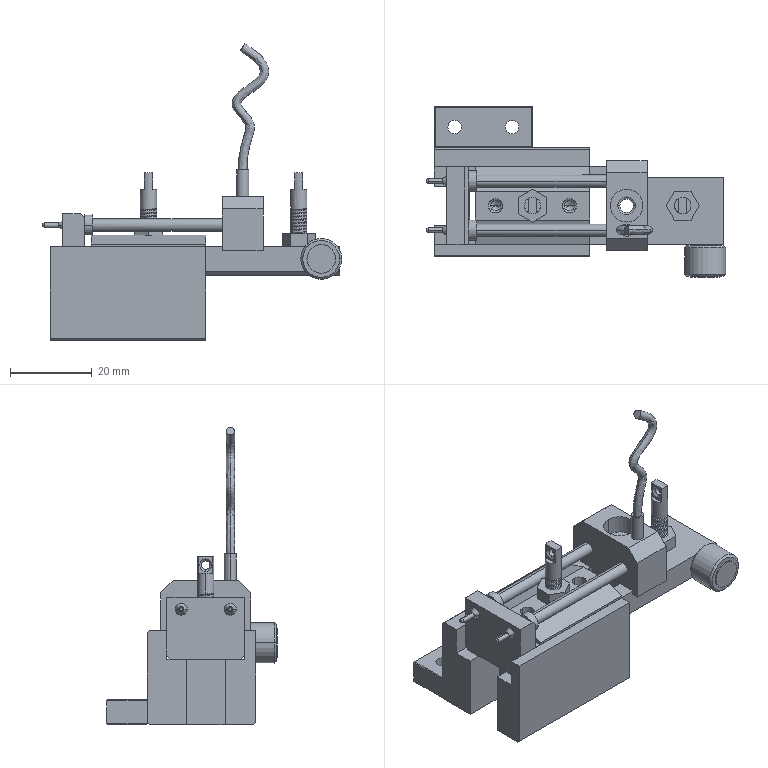Part | NX | 13 solids | 360 faces | box 73.15 x 41.75 x 72.548 mm | volume 31241 mm3 | cylinder 152 | plane 126 | cone 64 | spline 18 | commonest cylinder face diameters 4 x58 3 x28 3.3 x16 2.5 x14 3.5 x6 1 x4